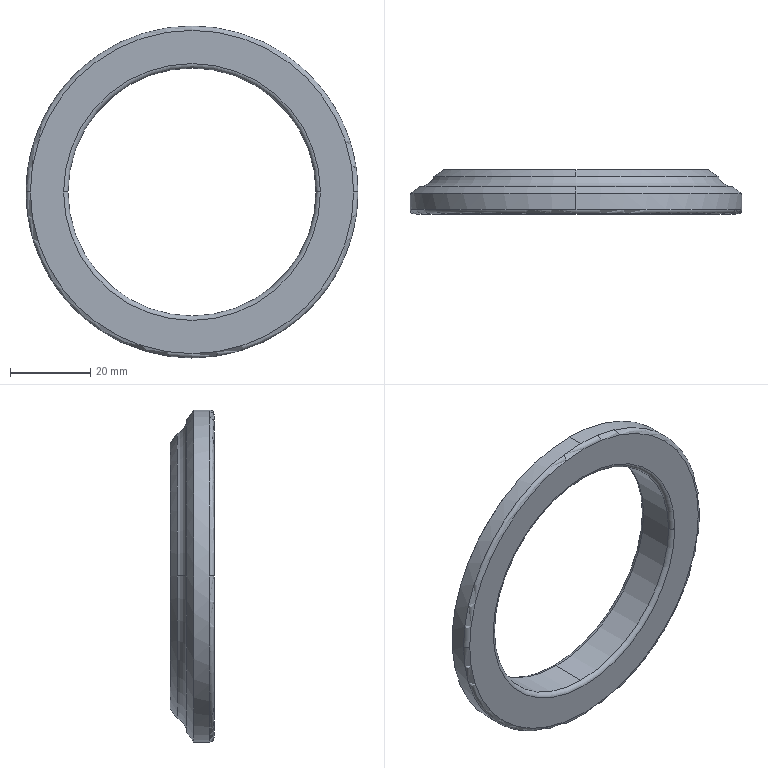Part | SolidWorks | features BaseBody 1 | 1 solid | 18 faces | box 83 x 11 x 83 mm | volume 19666 mm3 | torus 8 | cylinder 4 | cone 4 | plane 2 | commonest cylinder face diameters 62 x2 83 x2
STEP:
#1=CARTESIAN_POINT('',(-2100.85,891.097,-1577.624));
#2=VERTEX_POINT('',#1);
#3=CARTESIAN_POINT('',(-2165.05,891.097,-1577.624));
#4=VERTEX_POINT('',#3);
#5=CARTESIAN_POINT('',(-2132.95,891.097,-1577.624));
#6=DIRECTION('',(0.,-1.,0.));
#7=DIRECTION('',(1.,0.,0.));
#8=AXIS2_PLACEMENT_3D('',#5,#6,#7);
#9=CIRCLE('',#8,32.1);
#10=EDGE_CURVE('',#2,#4,#9,.T.);
#11=ORIENTED_EDGE('',*,*,#10,.F.);
#12=CARTESIAN_POINT('',(-2132.95,891.097,-1577.624));
#13=DIRECTION('',(0.,-1.,0.));
#14=DIRECTION('',(-1.,0.,0.));
#15=AXIS2_PLACEMENT_3D('',#12,#13,#14);
#16=CIRCLE('',#15,32.1);
#17=EDGE_CURVE('',#4,#2,#16,.T.);
#18=ORIENTED_EDGE('',*,*,#17,.F.);
#19=EDGE_LOOP('',(#11,#18));
#20=FACE_BOUND('',#19,.T.);
#21=CARTESIAN_POINT('',(-2092.55,891.097,-1577.624));
#22=VERTEX_POINT('',#21);
#23=CARTESIAN_POINT('',(-2173.35,891.097,-1577.624));
#24=VERTEX_POINT('',#23);
#25=CARTESIAN_POINT('',(-2132.95,891.097,-1577.624));
#26=DIRECTION('',(0.,-1.,0.));
#27=DIRECTION('',(1.,0.,0.));
#28=AXIS2_PLACEMENT_3D('',#25,#26,#27);
#29=CIRCLE('',#28,40.4);
#30=EDGE_CURVE('',#22,#24,#29,.T.);
#31=ORIENTED_EDGE('',*,*,#30,.T.);
#32=CARTESIAN_POINT('',(-2132.95,891.097,-1577.624));
#33=DIRECTION('',(0.,-1.,0.));
#34=DIRECTION('',(-1.,0.,0.));
#35=AXIS2_PLACEMENT_3D('',#32,#33,#34);
#36=CIRCLE('',#35,40.4);
#37=EDGE_CURVE('',#24,#22,#36,.T.);
#38=ORIENTED_EDGE('',*,*,#37,.T.);
#39=EDGE_LOOP('',(#31,#38));
#40=FACE_OUTER_BOUND('',#39,.T.);
#41=CARTESIAN_POINT('',(-2177.39,891.097,-1533.184));
#42=DIRECTION('',(0.,-1.,0.));
#43=DIRECTION('',(0.,0.,-1.));
#44=AXIS2_PLACEMENT_3D('',#41,#42,#43);
#45=PLANE('',#44);
#46=ADVANCED_FACE('',(#20,#40),#45,.T.);
#47=CARTESIAN_POINT('',(-2163.95,892.197,-1577.624));
#48=VERTEX_POINT('',#47);
#49=CARTESIAN_POINT('',(-2165.05,892.197,-1577.624));
#50=DIRECTION('',(0.,0.,-1.));
#51=DIRECTION('',(1.,0.,0.));
#52=AXIS2_PLACEMENT_3D('',#49,#50,#51);
#53=CIRCLE('',#52,1.1);
#54=EDGE_CURVE('',#48,#4,#53,.T.);
#55=ORIENTED_EDGE('',*,*,#54,.T.);
#56=ORIENTED_EDGE('',*,*,#17,.T.);
#57=CARTESIAN_POINT('',(-2101.95,892.197,-1577.624));
#58=VERTEX_POINT('',#57);
#59=CARTESIAN_POINT('',(-2100.85,892.197,-1577.624));
#60=DIRECTION('',(0.,0.,-1.));
#61=DIRECTION('',(0.,-1.,0.));
#62=AXIS2_PLACEMENT_3D('',#59,#60,#61);
#63=CIRCLE('',#62,1.1);
#64=EDGE_CURVE('',#2,#58,#63,.T.);
#65=ORIENTED_EDGE('',*,*,#64,.T.);
#66=CARTESIAN_POINT('',(-2132.95,892.197,-1608.624));
#67=VERTEX_POINT('',#66);
#68=CARTESIAN_POINT('',(-2132.95,892.197,-1577.624));
#69=DIRECTION('',(0.,1.,0.));
#70=DIRECTION('',(1.,0.,0.));
#71=AXIS2_PLACEMENT_3D('',#68,#69,#70);
#72=CIRCLE('',#71,31.);
#73=EDGE_CURVE('',#58,#67,#72,.T.);
#74=ORIENTED_EDGE('',*,*,#73,.T.);
#75=CARTESIAN_POINT('',(-2132.95,892.197,-1577.624));
#76=DIRECTION('',(0.,1.,0.));
#77=DIRECTION('',(0.,0.,-1.));
#78=AXIS2_PLACEMENT_3D('',#75,#76,#77);
#79=CIRCLE('',#78,31.);
#80=EDGE_CURVE('',#67,#48,#79,.T.);
#81=ORIENTED_EDGE('',*,*,#80,.T.);
#82=EDGE_LOOP('',(#55,#56,#65,#74,#81));
#83=FACE_OUTER_BOUND('',#82,.T.);
#84=CARTESIAN_POINT('',(-2132.95,892.197,-1577.624));
#85=DIRECTION('',(0.,1.,0.));
#86=DIRECTION('',(0.9962,0.,0.08716));
#87=AXIS2_PLACEMENT_3D('',#84,#85,#86);
#88=TOROIDAL_SURFACE('',#87,32.1,1.1);
#89=ADVANCED_FACE('',(#83),#88,.T.);
#90=CARTESIAN_POINT('',(-2132.95,892.197,-1546.624));
#91=VERTEX_POINT('',#90);
#92=CARTESIAN_POINT('',(-2132.95,900.997,-1546.624));
#93=VERTEX_POINT('',#92);
#94=CARTESIAN_POINT('',(-2132.95,892.197,-1546.624));
#95=DIRECTION('',(0.,1.,0.));
#96=VECTOR('',#95,1000.);
#97=LINE('',#94,#96);
#98=EDGE_CURVE('',#91,#93,#97,.T.);
#99=ORIENTED_EDGE('',*,*,#98,.T.);
#100=CARTESIAN_POINT('',(-2101.95,900.997,-1577.624));
#101=VERTEX_POINT('',#100);
#102=CARTESIAN_POINT('',(-2132.95,900.997,-1577.624));
#103=DIRECTION('',(0.,1.,0.));
#104=DIRECTION('',(0.,0.,1.));
#105=AXIS2_PLACEMENT_3D('',#102,#103,#104);
#106=CIRCLE('',#105,31.);
#107=EDGE_CURVE('',#93,#101,#106,.T.);
#108=ORIENTED_EDGE('',*,*,#107,.T.);
#109=CARTESIAN_POINT('',(-2132.95,900.997,-1608.624));
#110=VERTEX_POINT('',#109);
#111=CARTESIAN_POINT('',(-2132.95,900.997,-1577.624));
#112=DIRECTION('',(0.,1.,0.));
#113=DIRECTION('',(1.,0.,0.));
#114=AXIS2_PLACEMENT_3D('',#111,#112,#113);
#115=CIRCLE('',#114,31.);
#116=EDGE_CURVE('',#101,#110,#115,.T.);
#117=ORIENTED_EDGE('',*,*,#116,.T.);
#118=CARTESIAN_POINT('',(-2132.95,900.997,-1608.624));
#119=DIRECTION('',(0.,-1.,0.));
#120=VECTOR('',#119,1000.);
#121=LINE('',#118,#120);
#122=EDGE_CURVE('',#110,#67,#121,.T.);
#123=ORIENTED_EDGE('',*,*,#122,.T.);
#124=ORIENTED_EDGE('',*,*,#73,.F.);
#125=CARTESIAN_POINT('',(-2132.95,892.197,-1577.624));
#126=DIRECTION('',(0.,1.,0.));
#127=DIRECTION('',(0.,0.,1.));
#128=AXIS2_PLACEMENT_3D('',#125,#126,#127);
#129=CIRCLE('',#128,31.);
#130=EDGE_CURVE('',#91,#58,#129,.T.);
#131=ORIENTED_EDGE('',*,*,#130,.F.);
#132=EDGE_LOOP('',(#99,#108,#117,#123,#124,#131));
#133=FACE_OUTER_BOUND('',#132,.T.);
#134=CARTESIAN_POINT('',(-2132.95,901.437,-1577.624));
#135=DIRECTION('',(0.,-1.,0.));
#136=DIRECTION('',(-0.08716,0.,-0.9962));
#137=AXIS2_PLACEMENT_3D('',#134,#135,#136);
#138=CYLINDRICAL_SURFACE('',#137,31.);
#139=ADVANCED_FACE('',(#133),#138,.F.);
#140=CARTESIAN_POINT('',(-2165.05,902.097,-1577.624));
#141=VERTEX_POINT('',#140);
#142=CARTESIAN_POINT('',(-2163.95,900.997,-1577.624));
#143=VERTEX_POINT('',#142);
#144=CARTESIAN_POINT('',(-2165.05,900.997,-1577.624));
#145=DIRECTION('',(0.,0.,-1.));
#146=DIRECTION('',(0.,1.,0.));
#147=AXIS2_PLACEMENT_3D('',#144,#145,#146);
#148=CIRCLE('',#147,1.1);
#149=EDGE_CURVE('',#141,#143,#148,.T.);
#150=ORIENTED_EDGE('',*,*,#149,.T.);
#151=CARTESIAN_POINT('',(-2132.95,900.997,-1577.624));
#152=DIRECTION('',(0.,1.,0.));
#153=DIRECTION('',(0.,0.,-1.));
#154=AXIS2_PLACEMENT_3D('',#151,#152,#153);
#155=CIRCLE('',#154,31.);
#156=EDGE_CURVE('',#110,#143,#155,.T.);
#157=ORIENTED_EDGE('',*,*,#156,.F.);
#158=ORIENTED_EDGE('',*,*,#116,.F.);
#159=CARTESIAN_POINT('',(-2100.85,902.097,-1577.624));
#160=VERTEX_POINT('',#159);
#161=CARTESIAN_POINT('',(-2100.85,900.997,-1577.624));
#162=DIRECTION('',(0.,0.,-1.));
#163=DIRECTION('',(-1.,0.,0.));
#164=AXIS2_PLACEMENT_3D('',#161,#162,#163);
#165=CIRCLE('',#164,1.1);
#166=EDGE_CURVE('',#101,#160,#165,.T.);
#167=ORIENTED_EDGE('',*,*,#166,.T.);
#168=CARTESIAN_POINT('',(-2132.95,902.097,-1577.624));
#169=DIRECTION('',(0.,1.,0.));
#170=DIRECTION('',(1.,0.,0.));
#171=AXIS2_PLACEMENT_3D('',#168,#169,#170);
#172=CIRCLE('',#171,32.1);
#173=EDGE_CURVE('',#160,#141,#172,.T.);
#174=ORIENTED_EDGE('',*,*,#173,.T.);
#175=EDGE_LOOP('',(#150,#157,#158,#167,#174));
#176=FACE_OUTER_BOUND('',#175,.T.);
#177=CARTESIAN_POINT('',(-2132.95,900.997,-1577.624));
#178=DIRECTION('',(0.,1.,0.));
#179=DIRECTION('',(0.9962,0.,0.08716));
#180=AXIS2_PLACEMENT_3D('',#177,#178,#179);
#181=TOROIDAL_SURFACE('',#180,32.1,1.1);
#182=ADVANCED_FACE('',(#176),#181,.T.);
#183=CARTESIAN_POINT('',(-2132.95,902.097,-1577.624));
#184=DIRECTION('',(0.,1.,0.));
#185=DIRECTION('',(0.,0.,1.));
#186=AXIS2_PLACEMENT_3D('',#183,#184,#185);
#187=CIRCLE('',#186,32.1);
#188=EDGE_CURVE('',#141,#160,#187,.T.);
#189=ORIENTED_EDGE('',*,*,#188,.F.);
#190=ORIENTED_EDGE('',*,*,#173,.F.);
#191=EDGE_LOOP('',(#189,#190));
#192=FACE_BOUND('',#191,.T.);
#193=CARTESIAN_POINT('',(-2132.95,902.097,-1544.549));
#194=VERTEX_POINT('',#193);
#195=CARTESIAN_POINT('',(-2132.95,902.097,-1610.699));
#196=VERTEX_POINT('',#195);
#197=CARTESIAN_POINT('',(-2132.95,902.097,-1577.624));
#198=DIRECTION('',(0.,1.,0.));
#199=DIRECTION('',(0.,0.,1.));
#200=AXIS2_PLACEMENT_3D('',#197,#198,#199);
#201=CIRCLE('',#200,33.075);
#202=EDGE_CURVE('',#194,#196,#201,.T.);
#203=ORIENTED_EDGE('',*,*,#202,.T.);
#204=CARTESIAN_POINT('',(-2132.95,902.097,-1577.624));
#205=DIRECTION('',(0.,1.,0.));
#206=DIRECTION('',(0.,0.,-1.));
#207=AXIS2_PLACEMENT_3D('',#204,#205,#206);
#208=CIRCLE('',#207,33.075);
#209=EDGE_CURVE('',#196,#194,#208,.T.);
#210=ORIENTED_EDGE('',*,*,#209,.T.);
#211=EDGE_LOOP('',(#203,#210));
#212=FACE_OUTER_BOUND('',#211,.T.);
#213=CARTESIAN_POINT('',(-2169.332,902.097,-1614.007));
#214=DIRECTION('',(0.,1.,0.));
#215=DIRECTION('',(1.,0.,0.));
#216=AXIS2_PLACEMENT_3D('',#213,#214,#215);
#217=PLANE('',#216);
#218=ADVANCED_FACE('',(#192,#212),#217,.T.);
#219=CARTESIAN_POINT('',(-2132.95,900.346,-1542.049));
#220=VERTEX_POINT('',#219);
#221=CARTESIAN_POINT('',(-2132.95,900.346,-1542.049));
#222=DIRECTION('',(0.,0.5736,-0.8192));
#223=VECTOR('',#222,1000.);
#224=LINE('',#221,#223);
#225=EDGE_CURVE('',#220,#194,#224,.T.);
#226=ORIENTED_EDGE('',*,*,#225,.T.);
#227=ORIENTED_EDGE('',*,*,#209,.F.);
#228=CARTESIAN_POINT('',(-2132.95,900.346,-1613.2));
#229=VERTEX_POINT('',#228);
#230=CARTESIAN_POINT('',(-2132.95,902.097,-1610.699));
#231=DIRECTION('',(0.,-0.5736,-0.8192));
#232=VECTOR('',#231,1000.);
#233=LINE('',#230,#232);
#234=EDGE_CURVE('',#196,#229,#233,.T.);
#235=ORIENTED_EDGE('',*,*,#234,.T.);
#236=CARTESIAN_POINT('',(-2168.525,900.346,-1577.624));
#237=VERTEX_POINT('',#236);
#238=CARTESIAN_POINT('',(-2132.95,900.346,-1577.624));
#239=DIRECTION('',(0.,1.,0.));
#240=DIRECTION('',(0.,0.,-1.));
#241=AXIS2_PLACEMENT_3D('',#238,#239,#240);
#242=CIRCLE('',#241,35.576);
#243=EDGE_CURVE('',#229,#237,#242,.T.);
#244=ORIENTED_EDGE('',*,*,#243,.T.);
#245=CARTESIAN_POINT('',(-2132.95,900.346,-1577.624));
#246=DIRECTION('',(0.,1.,0.));
#247=DIRECTION('',(-1.,0.,0.));
#248=AXIS2_PLACEMENT_3D('',#245,#246,#247);
#249=CIRCLE('',#248,35.576);
#250=EDGE_CURVE('',#237,#220,#249,.T.);
#251=ORIENTED_EDGE('',*,*,#250,.T.);
#252=EDGE_LOOP('',(#226,#227,#235,#244,#251));
#253=FACE_OUTER_BOUND('',#252,.T.);
#254=CARTESIAN_POINT('',(-2132.95,902.184,-1577.624));
#255=DIRECTION('',(0.,-1.,0.));
#256=DIRECTION('',(0.08716,0.,0.9962));
#257=AXIS2_PLACEMENT_3D('',#254,#255,#256);
#258=CONICAL_SURFACE('',#257,32.95,0.9599);
#259=ADVANCED_FACE('',(#253),#258,.T.);
#260=CARTESIAN_POINT('',(-2093.854,897.881,-1577.624));
#261=VERTEX_POINT('',#260);
#262=CARTESIAN_POINT('',(-2097.374,900.346,-1577.624));
#263=VERTEX_POINT('',#262);
#264=CARTESIAN_POINT('',(-2093.7,901.847,-1577.624));
#265=DIRECTION('',(0.,0.,-1.));
#266=DIRECTION('',(-0.03878,-0.9992,0.));
#267=AXIS2_PLACEMENT_3D('',#264,#265,#266);
#268=CIRCLE('',#267,3.969);
#269=EDGE_CURVE('',#261,#263,#268,.T.);
#270=ORIENTED_EDGE('',*,*,#269,.T.);
#271=CARTESIAN_POINT('',(-2132.95,900.346,-1577.624));
#272=DIRECTION('',(0.,1.,0.));
#273=DIRECTION('',(0.,0.,1.));
#274=AXIS2_PLACEMENT_3D('',#271,#272,#273);
#275=CIRCLE('',#274,35.576);
#276=EDGE_CURVE('',#220,#263,#275,.T.);
#277=ORIENTED_EDGE('',*,*,#276,.F.);
#278=ORIENTED_EDGE('',*,*,#250,.F.);
#279=CARTESIAN_POINT('',(-2172.046,897.881,-1577.624));
#280=VERTEX_POINT('',#279);
#281=CARTESIAN_POINT('',(-2172.2,901.847,-1577.624));
#282=DIRECTION('',(0.,0.,-1.));
#283=DIRECTION('',(0.9257,-0.3782,0.));
#284=AXIS2_PLACEMENT_3D('',#281,#282,#283);
#285=CIRCLE('',#284,3.969);
#286=EDGE_CURVE('',#237,#280,#285,.T.);
#287=ORIENTED_EDGE('',*,*,#286,.T.);
#288=CARTESIAN_POINT('',(-2132.95,897.881,-1538.528));
#289=VERTEX_POINT('',#288);
#290=CARTESIAN_POINT('',(-2132.95,897.881,-1577.624));
#291=DIRECTION('',(0.,1.,0.));
#292=DIRECTION('',(-1.,0.,0.));
#293=AXIS2_PLACEMENT_3D('',#290,#291,#292);
#294=CIRCLE('',#293,39.096);
#295=EDGE_CURVE('',#280,#289,#294,.T.);
#296=ORIENTED_EDGE('',*,*,#295,.T.);
#297=CARTESIAN_POINT('',(-2132.95,897.881,-1577.624));
#298=DIRECTION('',(0.,1.,0.));
#299=DIRECTION('',(0.,0.,1.));
#300=AXIS2_PLACEMENT_3D('',#297,#298,#299);
#301=CIRCLE('',#300,39.096);
#302=EDGE_CURVE('',#289,#261,#301,.T.);
#303=ORIENTED_EDGE('',*,*,#302,.T.);
#304=EDGE_LOOP('',(#270,#277,#278,#287,#296,#303));
#305=FACE_OUTER_BOUND('',#304,.T.);
#306=CARTESIAN_POINT('',(-2132.95,901.847,-1577.624));
#307=DIRECTION('',(0.,1.,0.));
#308=DIRECTION('',(-0.9962,0.,-0.08716));
#309=AXIS2_PLACEMENT_3D('',#306,#307,#308);
#310=TOROIDAL_SURFACE('',#309,39.25,3.969);
#311=ADVANCED_FACE('',(#305),#310,.F.);
#312=CARTESIAN_POINT('',(-2132.95,896.197,-1536.124));
#313=VERTEX_POINT('',#312);
#314=CARTESIAN_POINT('',(-2132.95,896.197,-1536.124));
#315=DIRECTION('',(0.,0.5736,-0.8192));
#316=VECTOR('',#315,1000.);
#317=LINE('',#314,#316);
#318=EDGE_CURVE('',#313,#289,#317,.T.);
#319=ORIENTED_EDGE('',*,*,#318,.T.);
#320=ORIENTED_EDGE('',*,*,#295,.F.);
#321=CARTESIAN_POINT('',(-2132.95,897.881,-1616.721));
#322=VERTEX_POINT('',#321);
#323=CARTESIAN_POINT('',(-2132.95,897.881,-1577.624));
#324=DIRECTION('',(0.,1.,0.));
#325=DIRECTION('',(0.,0.,-1.));
#326=AXIS2_PLACEMENT_3D('',#323,#324,#325);
#327=CIRCLE('',#326,39.096);
#328=EDGE_CURVE('',#322,#280,#327,.T.);
#329=ORIENTED_EDGE('',*,*,#328,.F.);
#330=CARTESIAN_POINT('',(-2132.95,896.197,-1619.124));
#331=VERTEX_POINT('',#330);
#332=CARTESIAN_POINT('',(-2132.95,897.881,-1616.721));
#333=DIRECTION('',(0.,-0.5736,-0.8192));
#334=VECTOR('',#333,1000.);
#335=LINE('',#332,#334);
#336=EDGE_CURVE('',#322,#331,#335,.T.);
#337=ORIENTED_EDGE('',*,*,#336,.T.);
#338=CARTESIAN_POINT('',(-2132.95,896.197,-1577.624));
#339=DIRECTION('',(0.,1.,0.));
#340=DIRECTION('',(0.,0.,-1.));
#341=AXIS2_PLACEMENT_3D('',#338,#339,#340);
#342=CIRCLE('',#341,41.5);
#343=EDGE_CURVE('',#331,#313,#342,.T.);
#344=ORIENTED_EDGE('',*,*,#343,.T.);
#345=EDGE_LOOP('',(#319,#320,#329,#337,#344));
#346=FACE_OUTER_BOUND('',#345,.T.);
#347=CARTESIAN_POINT('',(-2132.95,897.965,-1577.624));
#348=DIRECTION('',(0.,-1.,0.));
#349=DIRECTION('',(0.08716,0.,0.9962));
#350=AXIS2_PLACEMENT_3D('',#347,#348,#349);
#351=CONICAL_SURFACE('',#350,38.976,0.9599);
#352=ADVANCED_FACE('',(#346),#351,.T.);
#353=CARTESIAN_POINT('',(-2132.95,892.197,-1536.124));
#354=VERTEX_POINT('',#353);
#355=CARTESIAN_POINT('',(-2132.95,892.197,-1536.124));
#356=DIRECTION('',(0.,1.,0.));
#357=VECTOR('',#356,1000.);
#358=LINE('',#355,#357);
#359=EDGE_CURVE('',#354,#313,#358,.T.);
#360=ORIENTED_EDGE('',*,*,#359,.T.);
#361=ORIENTED_EDGE('',*,*,#343,.F.);
#362=CARTESIAN_POINT('',(-2132.95,892.197,-1619.124));
#363=VERTEX_POINT('',#362);
#364=CARTESIAN_POINT('',(-2132.95,896.197,-1619.124));
#365=DIRECTION('',(0.,-1.,0.));
#366=VECTOR('',#365,1000.);
#367=LINE('',#364,#366);
#368=EDGE_CURVE('',#331,#363,#367,.T.);
#369=ORIENTED_EDGE('',*,*,#368,.T.);
#370=CARTESIAN_POINT('',(-2174.45,892.197,-1577.624));
#371=VERTEX_POINT('',#370);
#372=CARTESIAN_POINT('',(-2132.95,892.197,-1577.624));
#373=DIRECTION('',(0.,1.,0.));
#374=DIRECTION('',(0.,0.,-1.));
#375=AXIS2_PLACEMENT_3D('',#372,#373,#374);
#376=CIRCLE('',#375,41.5);
#377=EDGE_CURVE('',#363,#371,#376,.T.);
#378=ORIENTED_EDGE('',*,*,#377,.T.);
#379=CARTESIAN_POINT('',(-2132.95,892.197,-1577.624));
#380=DIRECTION('',(0.,1.,0.));
#381=DIRECTION('',(-1.,0.,0.));
#382=AXIS2_PLACEMENT_3D('',#379,#380,#381);
#383=CIRCLE('',#382,41.5);
#384=EDGE_CURVE('',#371,#354,#383,.T.);
#385=ORIENTED_EDGE('',*,*,#384,.T.);
#386=EDGE_LOOP('',(#360,#361,#369,#378,#385));
#387=FACE_OUTER_BOUND('',#386,.T.);
#388=CARTESIAN_POINT('',(-2132.95,891.997,-1577.624));
#389=DIRECTION('',(0.,-1.,0.));
#390=DIRECTION('',(0.08716,0.,0.9962));
#391=AXIS2_PLACEMENT_3D('',#388,#389,#390);
#392=CYLINDRICAL_SURFACE('',#391,41.5);
#393=ADVANCED_FACE('',(#387),#392,.T.);
#394=CARTESIAN_POINT('',(-2173.35,892.197,-1577.624));
#395=DIRECTION('',(0.,0.,-1.));
#396=DIRECTION('',(0.,-1.,0.));
#397=AXIS2_PLACEMENT_3D('',#394,#395,#396);
#398=CIRCLE('',#397,1.1);
#399=EDGE_CURVE('',#24,#371,#398,.T.);
#400=ORIENTED_EDGE('',*,*,#399,.T.);
#401=ORIENTED_EDGE('',*,*,#377,.F.);
#402=CARTESIAN_POINT('',(-2091.45,892.197,-1577.624));
#403=VERTEX_POINT('',#402);
#404=CARTESIAN_POINT('',(-2132.95,892.197,-1577.624));
#405=DIRECTION('',(0.,1.,0.));
#406=DIRECTION('',(1.,0.,0.));
#407=AXIS2_PLACEMENT_3D('',#404,#405,#406);
#408=CIRCLE('',#407,41.5);
#409=EDGE_CURVE('',#403,#363,#408,.T.);
#410=ORIENTED_EDGE('',*,*,#409,.F.);
#411=CARTESIAN_POINT('',(-2092.55,892.197,-1577.624));
#412=DIRECTION('',(0.,0.,-1.));
#413=DIRECTION('',(1.,0.,0.));
#414=AXIS2_PLACEMENT_3D('',#411,#412,#413);
#415=CIRCLE('',#414,1.1);
#416=EDGE_CURVE('',#403,#22,#415,.T.);
#417=ORIENTED_EDGE('',*,*,#416,.T.);
#418=ORIENTED_EDGE('',*,*,#37,.F.);
#419=EDGE_LOOP('',(#400,#401,#410,#417,#418));
#420=FACE_OUTER_BOUND('',#419,.T.);
#421=CARTESIAN_POINT('',(-2132.95,892.197,-1577.624));
#422=DIRECTION('',(0.,1.,0.));
#423=DIRECTION('',(0.9962,0.,0.08716));
#424=AXIS2_PLACEMENT_3D('',#421,#422,#423);
#425=TOROIDAL_SURFACE('',#424,40.4,1.1);
#426=ADVANCED_FACE('',(#420),#425,.T.);
#427=ORIENTED_EDGE('',*,*,#399,.F.);
#428=ORIENTED_EDGE('',*,*,#30,.F.);
#429=ORIENTED_EDGE('',*,*,#416,.F.);
#430=CARTESIAN_POINT('',(-2132.95,892.197,-1577.624));
#431=DIRECTION('',(0.,1.,0.));
#432=DIRECTION('',(0.,0.,1.));
#433=AXIS2_PLACEMENT_3D('',#430,#431,#432);
#434=CIRCLE('',#433,41.5);
#435=EDGE_CURVE('',#354,#403,#434,.T.);
#436=ORIENTED_EDGE('',*,*,#435,.F.);
#437=ORIENTED_EDGE('',*,*,#384,.F.);
#438=EDGE_LOOP('',(#427,#428,#429,#436,#437));
#439=FACE_OUTER_BOUND('',#438,.T.);
#440=CARTESIAN_POINT('',(-2132.95,892.197,-1577.624));
#441=DIRECTION('',(0.,1.,0.));
#442=DIRECTION('',(-0.9962,0.,-0.08716));
#443=AXIS2_PLACEMENT_3D('',#440,#441,#442);
#444=TOROIDAL_SURFACE('',#443,40.4,1.1);
#445=ADVANCED_FACE('',(#439),#444,.T.);
#446=ORIENTED_EDGE('',*,*,#359,.F.);
#447=ORIENTED_EDGE('',*,*,#435,.T.);
#448=ORIENTED_EDGE('',*,*,#409,.T.);
#449=ORIENTED_EDGE('',*,*,#368,.F.);
#450=CARTESIAN_POINT('',(-2132.95,896.197,-1577.624));
#451=DIRECTION('',(0.,1.,0.));
#452=DIRECTION('',(0.,0.,1.));
#453=AXIS2_PLACEMENT_3D('',#450,#451,#452);
#454=CIRCLE('',#453,41.5);
#455=EDGE_CURVE('',#313,#331,#454,.T.);
#456=ORIENTED_EDGE('',*,*,#455,.F.);
#457=EDGE_LOOP('',(#446,#447,#448,#449,#456));
#458=FACE_OUTER_BOUND('',#457,.T.);
#459=CARTESIAN_POINT('',(-2132.95,891.997,-1577.624));
#460=DIRECTION('',(0.,-1.,0.));
#461=DIRECTION('',(-0.08716,0.,-0.9962));
#462=AXIS2_PLACEMENT_3D('',#459,#460,#461);
#463=CYLINDRICAL_SURFACE('',#462,41.5);
#464=ADVANCED_FACE('',(#458),#463,.T.);
#465=ORIENTED_EDGE('',*,*,#318,.F.);
#466=ORIENTED_EDGE('',*,*,#455,.T.);
#467=ORIENTED_EDGE('',*,*,#336,.F.);
#468=CARTESIAN_POINT('',(-2132.95,897.881,-1577.624));
#469=DIRECTION('',(0.,1.,0.));
#470=DIRECTION('',(1.,0.,0.));
#471=AXIS2_PLACEMENT_3D('',#468,#469,#470);
#472=CIRCLE('',#471,39.096);
#473=EDGE_CURVE('',#261,#322,#472,.T.);
#474=ORIENTED_EDGE('',*,*,#473,.F.);
#475=ORIENTED_EDGE('',*,*,#302,.F.);
#476=EDGE_LOOP('',(#465,#466,#467,#474,#475));
#477=FACE_OUTER_BOUND('',#476,.T.);
#478=CARTESIAN_POINT('',(-2132.95,897.965,-1577.624));
#479=DIRECTION('',(0.,-1.,0.));
#480=DIRECTION('',(-0.08716,0.,-0.9962));
#481=AXIS2_PLACEMENT_3D('',#478,#479,#480);
#482=CONICAL_SURFACE('',#481,38.976,0.9599);
#483=ADVANCED_FACE('',(#477),#482,.T.);
#484=ORIENTED_EDGE('',*,*,#269,.F.);
#485=ORIENTED_EDGE('',*,*,#473,.T.);
#486=ORIENTED_EDGE('',*,*,#328,.T.);
#487=ORIENTED_EDGE('',*,*,#286,.F.);
#488=ORIENTED_EDGE('',*,*,#243,.F.);
#489=CARTESIAN_POINT('',(-2132.95,900.346,-1577.624));
#490=DIRECTION('',(0.,1.,0.));
#491=DIRECTION('',(1.,0.,0.));
#492=AXIS2_PLACEMENT_3D('',#489,#490,#491);
#493=CIRCLE('',#492,35.576);
#494=EDGE_CURVE('',#263,#229,#493,.T.);
#495=ORIENTED_EDGE('',*,*,#494,.F.);
#496=EDGE_LOOP('',(#484,#485,#486,#487,#488,#495));
#497=FACE_OUTER_BOUND('',#496,.T.);
#498=CARTESIAN_POINT('',(-2132.95,901.847,-1577.624));
#499=DIRECTION('',(0.,1.,0.));
#500=DIRECTION('',(0.9962,0.,0.08716));
#501=AXIS2_PLACEMENT_3D('',#498,#499,#500);
#502=TOROIDAL_SURFACE('',#501,39.25,3.969);
#503=ADVANCED_FACE('',(#497),#502,.F.);
#504=ORIENTED_EDGE('',*,*,#225,.F.);
#505=ORIENTED_EDGE('',*,*,#276,.T.);
#506=ORIENTED_EDGE('',*,*,#494,.T.);
#507=ORIENTED_EDGE('',*,*,#234,.F.);
#508=ORIENTED_EDGE('',*,*,#202,.F.);
#509=EDGE_LOOP('',(#504,#505,#506,#507,#508));
#510=FACE_OUTER_BOUND('',#509,.T.);
#511=CARTESIAN_POINT('',(-2132.95,902.184,-1577.624));
#512=DIRECTION('',(0.,-1.,0.));
#513=DIRECTION('',(-0.08716,0.,-0.9962));
#514=AXIS2_PLACEMENT_3D('',#511,#512,#513);
#515=CONICAL_SURFACE('',#514,32.95,0.9599);
#516=ADVANCED_FACE('',(#510),#515,.T.);
#517=ORIENTED_EDGE('',*,*,#149,.F.);
#518=ORIENTED_EDGE('',*,*,#188,.T.);
#519=ORIENTED_EDGE('',*,*,#166,.F.);
#520=ORIENTED_EDGE('',*,*,#107,.F.);
#521=CARTESIAN_POINT('',(-2132.95,900.997,-1577.624));
#522=DIRECTION('',(0.,1.,0.));
#523=DIRECTION('',(-1.,0.,0.));
#524=AXIS2_PLACEMENT_3D('',#521,#522,#523);
#525=CIRCLE('',#524,31.);
#526=EDGE_CURVE('',#143,#93,#525,.T.);
#527=ORIENTED_EDGE('',*,*,#526,.F.);
#528=EDGE_LOOP('',(#517,#518,#519,#520,#527));
#529=FACE_OUTER_BOUND('',#528,.T.);
#530=CARTESIAN_POINT('',(-2132.95,900.997,-1577.624));
#531=DIRECTION('',(0.,1.,0.));
#532=DIRECTION('',(-0.9962,0.,-0.08716));
#533=AXIS2_PLACEMENT_3D('',#530,#531,#532);
#534=TOROIDAL_SURFACE('',#533,32.1,1.1);
#535=ADVANCED_FACE('',(#529),#534,.T.);
#536=ORIENTED_EDGE('',*,*,#98,.F.);
#537=CARTESIAN_POINT('',(-2132.95,892.197,-1577.624));
#538=DIRECTION('',(0.,1.,0.));
#539=DIRECTION('',(-1.,0.,0.));
#540=AXIS2_PLACEMENT_3D('',#537,#538,#539);
#541=CIRCLE('',#540,31.);
#542=EDGE_CURVE('',#48,#91,#541,.T.);
#543=ORIENTED_EDGE('',*,*,#542,.F.);
#544=ORIENTED_EDGE('',*,*,#80,.F.);
#545=ORIENTED_EDGE('',*,*,#122,.F.);
#546=ORIENTED_EDGE('',*,*,#156,.T.);
#547=ORIENTED_EDGE('',*,*,#526,.T.);
#548=EDGE_LOOP('',(#536,#543,#544,#545,#546,#547));
#549=FACE_OUTER_BOUND('',#548,.T.);
#550=CARTESIAN_POINT('',(-2132.95,901.437,-1577.624));
#551=DIRECTION('',(0.,-1.,0.));
#552=DIRECTION('',(0.08716,0.,0.9962));
#553=AXIS2_PLACEMENT_3D('',#550,#551,#552);
#554=CYLINDRICAL_SURFACE('',#553,31.);
#555=ADVANCED_FACE('',(#549),#554,.F.);
#556=ORIENTED_EDGE('',*,*,#54,.F.);
#557=ORIENTED_EDGE('',*,*,#542,.T.);
#558=ORIENTED_EDGE('',*,*,#130,.T.);
#559=ORIENTED_EDGE('',*,*,#64,.F.);
#560=ORIENTED_EDGE('',*,*,#10,.T.);
#561=EDGE_LOOP('',(#556,#557,#558,#559,#560));
#562=FACE_OUTER_BOUND('',#561,.T.);
#563=CARTESIAN_POINT('',(-2132.95,892.197,-1577.624));
#564=DIRECTION('',(0.,1.,0.));
#565=DIRECTION('',(-0.9962,0.,-0.08716));
#566=AXIS2_PLACEMENT_3D('',#563,#564,#565);
#567=TOROIDAL_SURFACE('',#566,32.1,1.1);
#568=ADVANCED_FACE('',(#562),#567,.T.);
#569=CLOSED_SHELL('',(#46,#89,#139,#182,#218,#259,#311,#352,#393,#426,#445,#464,#483,#503,#516,#535,#555,#568));
#570=MANIFOLD_SOLID_BREP('',#569);
#571=CARTESIAN_POINT('',(0.,0.,0.));
#572=DIRECTION('',(0.,0.,1.));
#573=DIRECTION('',(1.,0.,0.));
#574=AXIS2_PLACEMENT_3D('',#571,#572,#573);
#575=(LENGTH_UNIT()NAMED_UNIT(*)SI_UNIT(.MILLI.,.METRE.));
#576=UNCERTAINTY_MEASURE_WITH_UNIT(LENGTH_MEASURE(0.00001),#575,'','');
#577=(NAMED_UNIT(*)PLANE_ANGLE_UNIT()SI_UNIT($,.RADIAN.));
#578=(NAMED_UNIT(*)SI_UNIT($,.STERADIAN.)SOLID_ANGLE_UNIT());
#579=(GEOMETRIC_REPRESENTATION_CONTEXT(3)GLOBAL_UNCERTAINTY_ASSIGNED_CONTEXT((#576))GLOBAL_UNIT_ASSIGNED_CONTEXT((#575,#577,#578))REPRESENTATION_CONTEXT('',''));
#580=ADVANCED_BREP_SHAPE_REPRESENTATION('',(#570,#574),#579);